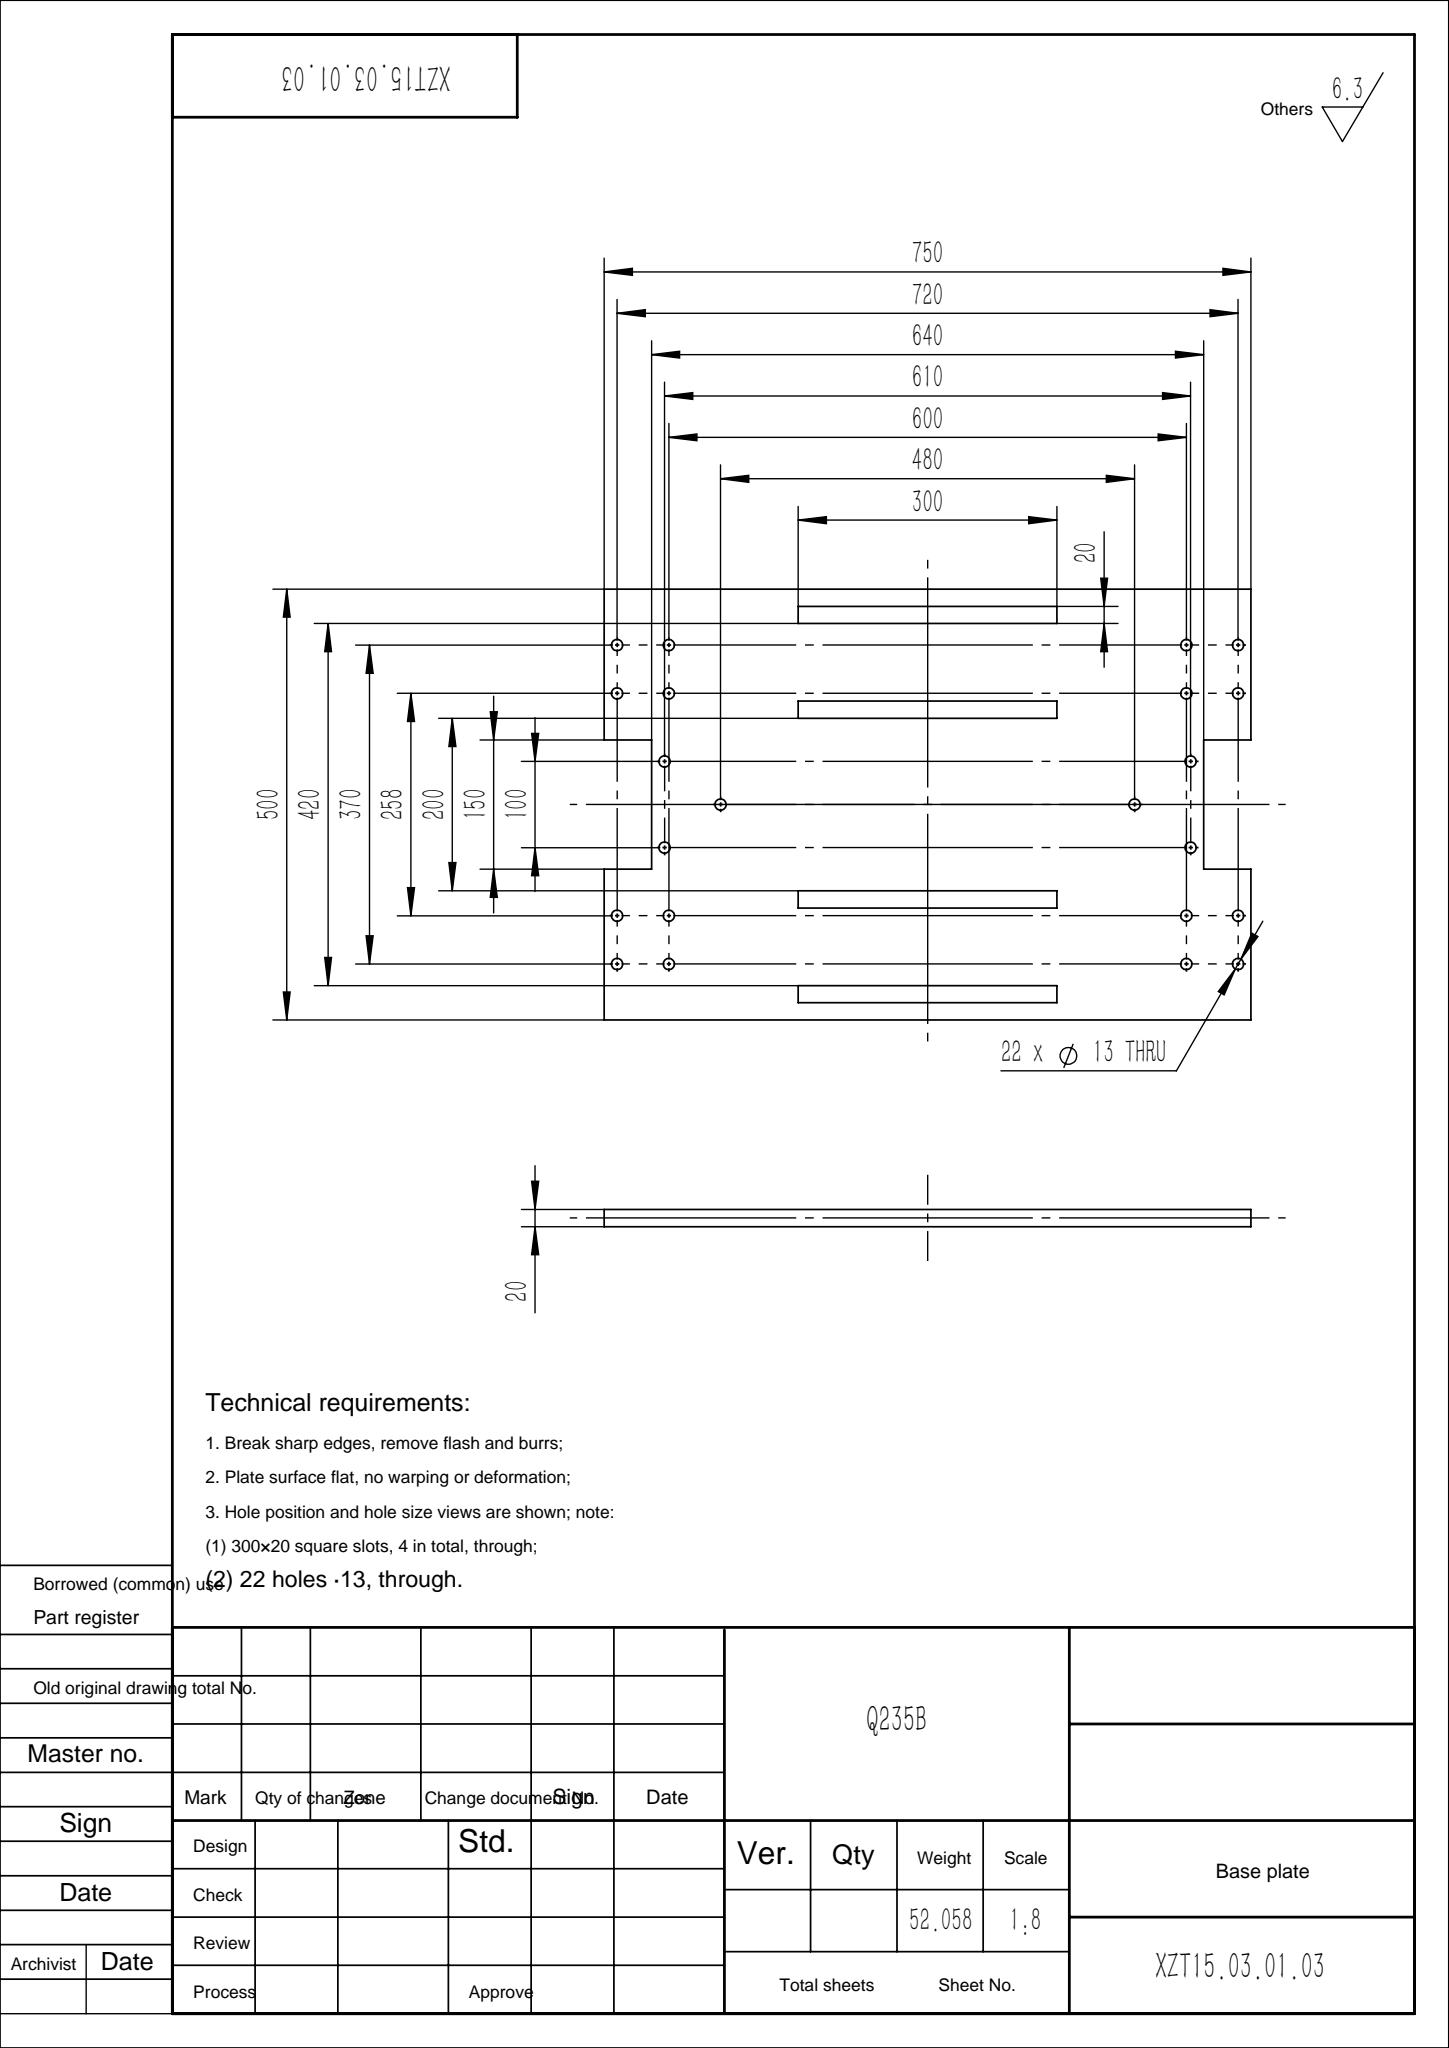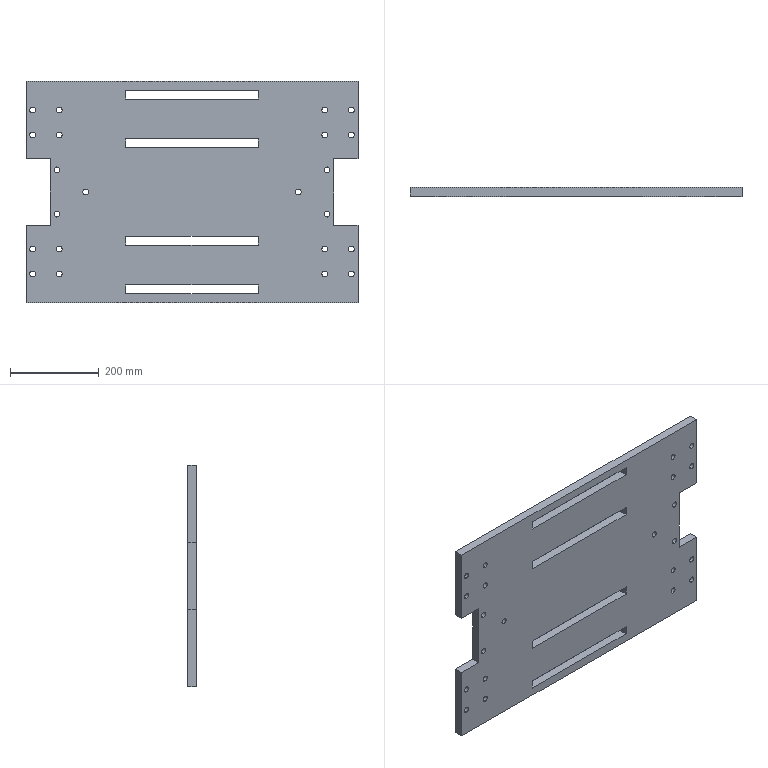Part | SolidWorks | features Extrusion 1, HoleWzd 1 | 1 solid | 74 faces | box 750 x 20 x 500 mm | volume 6631598 mm3 | cylinder 44 | plane 30 | commonest cylinder face diameters 13 x44